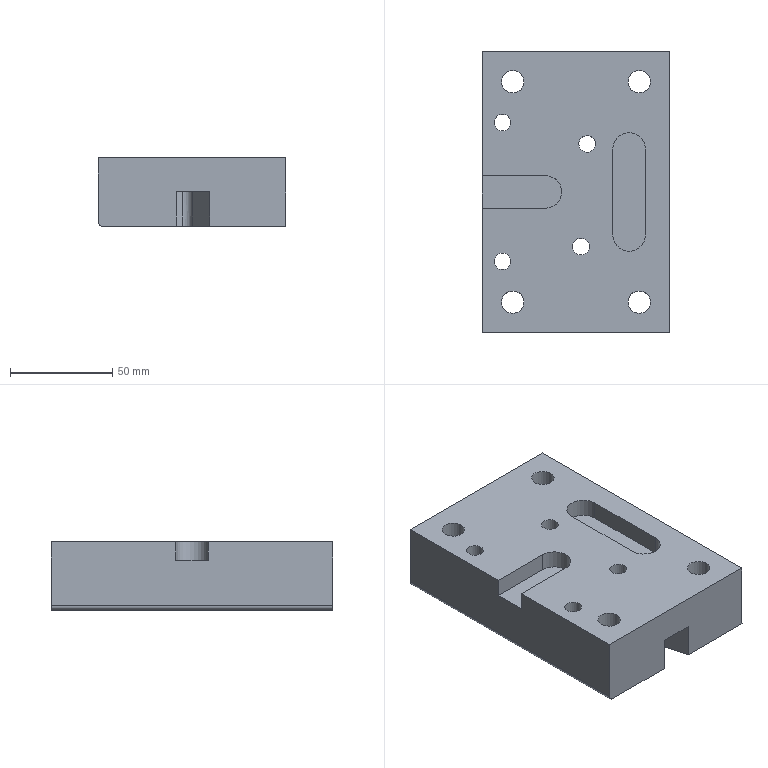Part | STEP file | gslz 2016.10.28-6_id42_x_t | 1 solid | 83 faces | box 92 x 138 x 33.5 mm | volume 323745 mm3 | plane 39 | cylinder 36 | cone 4 | torus 4 | commonest cylinder face diameters 8 x8 4.5 x5 8.2 x4 10 x4 11 x4 17 x4